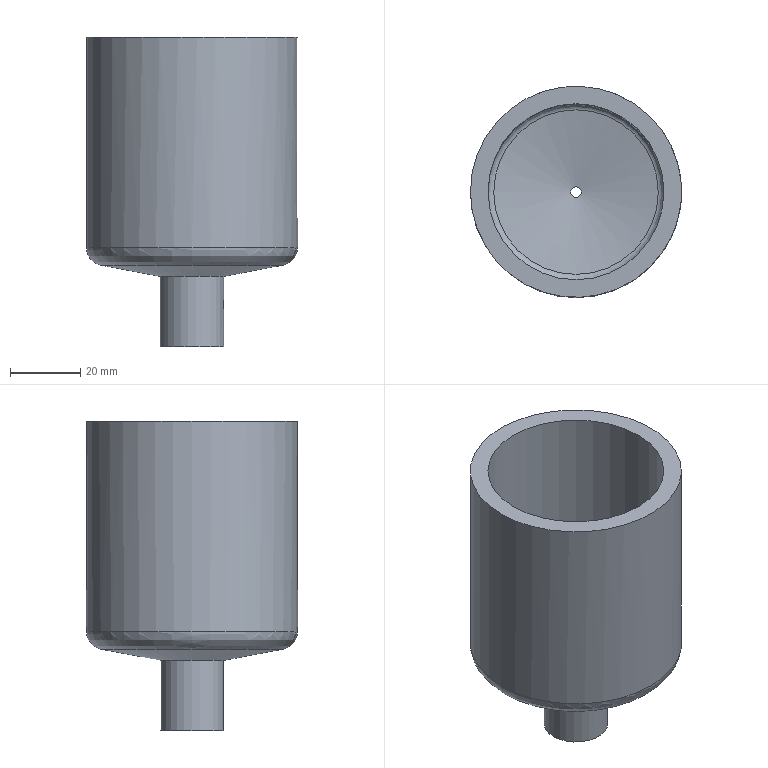Part | NX | features CYLINDER 3, BLEND 2, DATUM_CSYS 2, HOLE PACKAGE 2, SIMPLE HOLE 2, SYMBOLIC_THREAD 2, SKETCH 1, SWP104 1 | 1 solid | 18 faces | box 60 x 60 x 88 mm | volume 68833 mm3 | cylinder 8 | cone 4 | plane 4 | torus 2 | commonest cylinder face diameters 3 x2 8.5 x1 8.7 x1 12 x1 18 x1 50 x1
STEP:
#1=CARTESIAN_POINT('',(30.,0.,28.138));
#2=VERTEX_POINT('',#1);
#3=CARTESIAN_POINT('',(0.,0.,28.138));
#4=DIRECTION('',(0.,0.,1.));
#5=DIRECTION('',(1.,0.,0.));
#6=AXIS2_PLACEMENT_3D('',#3,#4,#5);
#7=CIRCLE('',#6,30.);
#8=EDGE_CURVE('',#2,#2,#7,.T.);
#9=ORIENTED_EDGE('',*,*,#8,.T.);
#10=EDGE_LOOP('',(#9));
#11=FACE_BOUND('',#10,.T.);
#12=CARTESIAN_POINT('',(-30.,0.,88.));
#13=VERTEX_POINT('',#12);
#14=CARTESIAN_POINT('',(0.,0.,88.));
#15=DIRECTION('',(0.,0.,-1.));
#16=DIRECTION('',(-1.,0.,0.));
#17=AXIS2_PLACEMENT_3D('',#14,#15,#16);
#18=CIRCLE('',#17,30.);
#19=EDGE_CURVE('',#13,#13,#18,.T.);
#20=ORIENTED_EDGE('',*,*,#19,.T.);
#21=EDGE_LOOP('',(#20));
#22=FACE_BOUND('',#21,.T.);
#23=CARTESIAN_POINT('',(0.,0.,0.));
#24=DIRECTION('',(0.,0.,-1.));
#25=DIRECTION('',(-1.,0.,0.));
#26=AXIS2_PLACEMENT_3D('',#23,#24,#25);
#27=CYLINDRICAL_SURFACE('',#26,30.);
#28=ADVANCED_FACE('',(#11,#22),#27,.T.);
#29=CARTESIAN_POINT('',(-25.936,0.,23.226));
#30=VERTEX_POINT('',#29);
#31=CARTESIAN_POINT('',(0.,0.,23.226));
#32=DIRECTION('',(0.,0.,-1.));
#33=DIRECTION('',(-1.,0.,0.));
#34=AXIS2_PLACEMENT_3D('',#31,#32,#33);
#35=CIRCLE('',#34,25.936);
#36=EDGE_CURVE('',#30,#30,#35,.T.);
#37=ORIENTED_EDGE('',*,*,#36,.T.);
#38=EDGE_LOOP('',(#37));
#39=FACE_BOUND('',#38,.T.);
#40=CARTESIAN_POINT('',(-9.,0.,20.));
#41=VERTEX_POINT('',#40);
#42=CARTESIAN_POINT('',(0.,0.,20.));
#43=DIRECTION('',(0.,0.,-1.));
#44=DIRECTION('',(-1.,0.,0.));
#45=AXIS2_PLACEMENT_3D('',#42,#43,#44);
#46=CIRCLE('',#45,9.);
#47=EDGE_CURVE('',#41,#41,#46,.T.);
#48=ORIENTED_EDGE('',*,*,#47,.F.);
#49=EDGE_LOOP('',(#48));
#50=FACE_BOUND('',#49,.T.);
#51=CARTESIAN_POINT('',(0.,0.,24.));
#52=DIRECTION('',(0.,0.,1.));
#53=DIRECTION('',(1.,0.,0.));
#54=AXIS2_PLACEMENT_3D('',#51,#52,#53);
#55=CONICAL_SURFACE('',#54,30.,1.383);
#56=ADVANCED_FACE('',(#39,#50),#55,.T.);
#57=CARTESIAN_POINT('',(9.,0.,10.5));
#58=VERTEX_POINT('',#57);
#59=CARTESIAN_POINT('',(8.937,1.177,10.826));
#60=CARTESIAN_POINT('',(9.031,-0.0002785,10.337));
#61=CARTESIAN_POINT('',(8.937,-1.176,10.825));
#62=CARTESIAN_POINT('',(8.842,-1.662,11.999));
#63=CARTESIAN_POINT('',(8.937,-1.176,13.175));
#64=CARTESIAN_POINT('',(9.031,-0.00044,13.662));
#65=CARTESIAN_POINT('',(8.938,1.174,13.177));
#66=CARTESIAN_POINT('',(8.842,1.662,12.001));
#67=CARTESIAN_POINT('',(8.937,1.177,10.826));
#68=CARTESIAN_POINT('',(9.031,-0.0002785,10.337));
#69=CARTESIAN_POINT('',(8.937,-1.176,10.825));
#70=B_SPLINE_CURVE_WITH_KNOTS('',3,(#59,#60,#61,#62,#63,#64,#65,#66,#67,#68,#69),.UNSPECIFIED.,.T.,.F.,(1,1,1,1,1,1,1,1,1,1,1,1,1,1,1),(-0.003523,-0.002349,-0.001174,0.,0.001174,0.002349,0.003523,0.004697,0.005872,0.007046,0.00822,0.009395,0.01057,0.01174,0.01292),.UNSPECIFIED.);
#71=EDGE_CURVE('',#58,#58,#70,.T.);
#72=ORIENTED_EDGE('',*,*,#71,.T.);
#73=EDGE_LOOP('',(#72));
#74=FACE_BOUND('',#73,.T.);
#75=CARTESIAN_POINT('',(-9.,0.,0.));
#76=VERTEX_POINT('',#75);
#77=CARTESIAN_POINT('',(0.,0.,0.));
#78=DIRECTION('',(0.,0.,-1.));
#79=DIRECTION('',(-1.,0.,0.));
#80=AXIS2_PLACEMENT_3D('',#77,#78,#79);
#81=CIRCLE('',#80,9.);
#82=EDGE_CURVE('',#76,#76,#81,.T.);
#83=ORIENTED_EDGE('',*,*,#82,.F.);
#84=EDGE_LOOP('',(#83));
#85=FACE_BOUND('',#84,.T.);
#86=ORIENTED_EDGE('',*,*,#47,.T.);
#87=EDGE_LOOP('',(#86));
#88=FACE_BOUND('',#87,.T.);
#89=CARTESIAN_POINT('',(0.,0.,0.));
#90=DIRECTION('',(0.,0.,-1.));
#91=DIRECTION('',(-1.,0.,0.));
#92=AXIS2_PLACEMENT_3D('',#89,#90,#91);
#93=CYLINDRICAL_SURFACE('',#92,9.);
#94=ADVANCED_FACE('',(#74,#85,#88),#93,.T.);
#95=CARTESIAN_POINT('',(5.,0.,0.));
#96=VERTEX_POINT('',#95);
#97=CARTESIAN_POINT('',(0.,0.,0.));
#98=DIRECTION('',(0.,0.,1.));
#99=DIRECTION('',(1.,0.,0.));
#100=AXIS2_PLACEMENT_3D('',#97,#98,#99);
#101=CIRCLE('',#100,5.);
#102=EDGE_CURVE('',#96,#96,#101,.T.);
#103=ORIENTED_EDGE('',*,*,#102,.T.);
#104=EDGE_LOOP('',(#103));
#105=FACE_BOUND('',#104,.T.);
#106=ORIENTED_EDGE('',*,*,#82,.T.);
#107=EDGE_LOOP('',(#106));
#108=FACE_BOUND('',#107,.T.);
#109=CARTESIAN_POINT('',(0.,9.,0.));
#110=DIRECTION('',(0.,0.,1.));
#111=DIRECTION('',(1.,0.,0.));
#112=AXIS2_PLACEMENT_3D('',#109,#110,#111);
#113=PLANE('',#112);
#114=ADVANCED_FACE('',(#105,#108),#113,.F.);
#115=CARTESIAN_POINT('',(23.374,0.,27.828));
#116=VERTEX_POINT('',#115);
#117=CARTESIAN_POINT('',(0.,0.,27.828));
#118=DIRECTION('',(0.,0.,1.));
#119=DIRECTION('',(1.,0.,0.));
#120=AXIS2_PLACEMENT_3D('',#117,#118,#119);
#121=CIRCLE('',#120,23.374);
#122=EDGE_CURVE('',#116,#116,#121,.T.);
#123=ORIENTED_EDGE('',*,*,#122,.T.);
#124=EDGE_LOOP('',(#123));
#125=FACE_BOUND('',#124,.T.);
#126=CARTESIAN_POINT('',(1.5,0.,23.661));
#127=VERTEX_POINT('',#126);
#128=CARTESIAN_POINT('',(0.,0.,23.661));
#129=DIRECTION('',(0.,0.,1.));
#130=DIRECTION('',(1.,0.,0.));
#131=AXIS2_PLACEMENT_3D('',#128,#129,#130);
#132=CIRCLE('',#131,1.5);
#133=EDGE_CURVE('',#127,#127,#132,.F.);
#134=ORIENTED_EDGE('',*,*,#133,.T.);
#135=EDGE_LOOP('',(#134));
#136=FACE_BOUND('',#135,.T.);
#137=CARTESIAN_POINT('',(0.,0.,23.376));
#138=DIRECTION('',(0.,0.,1.));
#139=DIRECTION('',(1.,0.,0.));
#140=AXIS2_PLACEMENT_3D('',#137,#138,#139);
#141=CONICAL_SURFACE('',#140,0.,1.383);
#142=ADVANCED_FACE('',(#125,#136),#141,.F.);
#143=CARTESIAN_POINT('',(-25.,0.,29.793));
#144=VERTEX_POINT('',#143);
#145=CARTESIAN_POINT('',(0.,0.,29.793));
#146=DIRECTION('',(0.,0.,-1.));
#147=DIRECTION('',(-1.,0.,0.));
#148=AXIS2_PLACEMENT_3D('',#145,#146,#147);
#149=CIRCLE('',#148,25.);
#150=EDGE_CURVE('',#144,#144,#149,.T.);
#151=ORIENTED_EDGE('',*,*,#150,.T.);
#152=EDGE_LOOP('',(#151));
#153=FACE_BOUND('',#152,.T.);
#154=CARTESIAN_POINT('',(-25.,0.,88.));
#155=VERTEX_POINT('',#154);
#156=CARTESIAN_POINT('',(0.,0.,88.));
#157=DIRECTION('',(0.,0.,-1.));
#158=DIRECTION('',(-1.,0.,0.));
#159=AXIS2_PLACEMENT_3D('',#156,#157,#158);
#160=CIRCLE('',#159,25.);
#161=EDGE_CURVE('',#155,#155,#160,.T.);
#162=ORIENTED_EDGE('',*,*,#161,.F.);
#163=EDGE_LOOP('',(#162));
#164=FACE_BOUND('',#163,.T.);
#165=CARTESIAN_POINT('',(0.,0.,0.));
#166=DIRECTION('',(0.,0.,-1.));
#167=DIRECTION('',(-1.,0.,0.));
#168=AXIS2_PLACEMENT_3D('',#165,#166,#167);
#169=CYLINDRICAL_SURFACE('',#168,25.);
#170=ADVANCED_FACE('',(#153,#164),#169,.F.);
#171=ORIENTED_EDGE('',*,*,#19,.F.);
#172=EDGE_LOOP('',(#171));
#173=FACE_BOUND('',#172,.T.);
#174=ORIENTED_EDGE('',*,*,#161,.T.);
#175=EDGE_LOOP('',(#174));
#176=FACE_BOUND('',#175,.T.);
#177=CARTESIAN_POINT('',(0.,25.,88.));
#178=DIRECTION('',(0.,0.,-1.));
#179=DIRECTION('',(-1.,0.,0.));
#180=AXIS2_PLACEMENT_3D('',#177,#178,#179);
#181=PLANE('',#180);
#182=ADVANCED_FACE('',(#173,#176),#181,.F.);
#183=CARTESIAN_POINT('',(4.25,0.,0.75));
#184=VERTEX_POINT('',#183);
#185=CARTESIAN_POINT('',(0.,0.,0.75));
#186=DIRECTION('',(0.,0.,1.));
#187=DIRECTION('',(1.,0.,0.));
#188=AXIS2_PLACEMENT_3D('',#185,#186,#187);
#189=CIRCLE('',#188,4.25);
#190=EDGE_CURVE('',#184,#184,#189,.F.);
#191=ORIENTED_EDGE('',*,*,#190,.T.);
#192=EDGE_LOOP('',(#191));
#193=FACE_BOUND('',#192,.T.);
#194=CARTESIAN_POINT('',(-4.25,0.,10.));
#195=VERTEX_POINT('',#194);
#196=CARTESIAN_POINT('',(0.,0.,10.));
#197=DIRECTION('',(0.,0.,-1.));
#198=DIRECTION('',(-1.,0.,0.));
#199=AXIS2_PLACEMENT_3D('',#196,#197,#198);
#200=CIRCLE('',#199,4.25);
#201=EDGE_CURVE('',#195,#195,#200,.F.);
#202=ORIENTED_EDGE('',*,*,#201,.T.);
#203=EDGE_LOOP('',(#202));
#204=FACE_BOUND('',#203,.T.);
#205=CARTESIAN_POINT('',(0.,0.,0.));
#206=DIRECTION('',(0.,0.,1.));
#207=DIRECTION('',(1.,0.,0.));
#208=AXIS2_PLACEMENT_3D('',#205,#206,#207);
#209=CYLINDRICAL_SURFACE('',#208,4.25);
#210=ADVANCED_FACE('',(#193,#204),#209,.F.);
#211=ORIENTED_EDGE('',*,*,#190,.F.);
#212=EDGE_LOOP('',(#211));
#213=FACE_BOUND('',#212,.T.);
#214=ORIENTED_EDGE('',*,*,#102,.F.);
#215=EDGE_LOOP('',(#214));
#216=FACE_BOUND('',#215,.T.);
#217=CARTESIAN_POINT('',(0.,0.,0.));
#218=DIRECTION('',(0.,0.,-1.));
#219=DIRECTION('',(-1.,0.,0.));
#220=AXIS2_PLACEMENT_3D('',#217,#218,#219);
#221=CONICAL_SURFACE('',#220,5.,0.7854);
#222=ADVANCED_FACE('',(#213,#216),#221,.F.);
#223=CARTESIAN_POINT('',(6.,0.,10.));
#224=VERTEX_POINT('',#223);
#225=CARTESIAN_POINT('',(0.,0.,10.));
#226=DIRECTION('',(0.,0.,1.));
#227=DIRECTION('',(1.,0.,0.));
#228=AXIS2_PLACEMENT_3D('',#225,#226,#227);
#229=CIRCLE('',#228,6.);
#230=EDGE_CURVE('',#224,#224,#229,.T.);
#231=ORIENTED_EDGE('',*,*,#230,.T.);
#232=EDGE_LOOP('',(#231));
#233=FACE_BOUND('',#232,.T.);
#234=ORIENTED_EDGE('',*,*,#201,.F.);
#235=EDGE_LOOP('',(#234));
#236=FACE_BOUND('',#235,.T.);
#237=CARTESIAN_POINT('',(0.,0.,10.));
#238=DIRECTION('',(0.,0.,-1.));
#239=DIRECTION('',(-1.,0.,0.));
#240=AXIS2_PLACEMENT_3D('',#237,#238,#239);
#241=PLANE('',#240);
#242=ADVANCED_FACE('',(#233,#236),#241,.F.);
#243=CARTESIAN_POINT('',(4.35,0.,14.));
#244=VERTEX_POINT('',#243);
#245=CARTESIAN_POINT('',(0.,0.,14.));
#246=DIRECTION('',(0.,0.,1.));
#247=DIRECTION('',(1.,0.,0.));
#248=AXIS2_PLACEMENT_3D('',#245,#246,#247);
#249=CIRCLE('',#248,4.35);
#250=EDGE_CURVE('',#244,#244,#249,.T.);
#251=ORIENTED_EDGE('',*,*,#250,.T.);
#252=EDGE_LOOP('',(#251));
#253=FACE_BOUND('',#252,.T.);
#254=CARTESIAN_POINT('',(-6.,0.,14.));
#255=VERTEX_POINT('',#254);
#256=CARTESIAN_POINT('',(0.,0.,14.));
#257=DIRECTION('',(0.,0.,-1.));
#258=DIRECTION('',(-1.,0.,0.));
#259=AXIS2_PLACEMENT_3D('',#256,#257,#258);
#260=CIRCLE('',#259,6.);
#261=EDGE_CURVE('',#255,#255,#260,.T.);
#262=ORIENTED_EDGE('',*,*,#261,.T.);
#263=EDGE_LOOP('',(#262));
#264=FACE_BOUND('',#263,.T.);
#265=CARTESIAN_POINT('',(0.,0.,14.));
#266=DIRECTION('',(0.,0.,1.));
#267=DIRECTION('',(1.,0.,0.));
#268=AXIS2_PLACEMENT_3D('',#265,#266,#267);
#269=PLANE('',#268);
#270=ADVANCED_FACE('',(#253,#264),#269,.F.);
#271=CARTESIAN_POINT('',(6.,0.,10.5));
#272=VERTEX_POINT('',#271);
#273=CARTESIAN_POINT('',(5.906,-1.177,10.826));
#274=CARTESIAN_POINT('',(6.047,0.0002147,10.337));
#275=CARTESIAN_POINT('',(5.906,1.176,10.825));
#276=CARTESIAN_POINT('',(5.761,1.662,11.998));
#277=CARTESIAN_POINT('',(5.906,1.175,13.176));
#278=CARTESIAN_POINT('',(6.047,0.0007133,13.662));
#279=CARTESIAN_POINT('',(5.906,-1.174,13.176));
#280=CARTESIAN_POINT('',(5.761,-1.662,12.001));
#281=CARTESIAN_POINT('',(5.906,-1.177,10.826));
#282=CARTESIAN_POINT('',(6.047,0.0002147,10.337));
#283=CARTESIAN_POINT('',(5.906,1.176,10.825));
#284=B_SPLINE_CURVE_WITH_KNOTS('',3,(#273,#274,#275,#276,#277,#278,#279,#280,#281,#282,#283),.UNSPECIFIED.,.T.,.F.,(1,1,1,1,1,1,1,1,1,1,1,1,1,1,1),(-0.003531,-0.002354,-0.001177,0.,0.001177,0.002354,0.003531,0.004708,0.005885,0.007062,0.008239,0.009416,0.01059,0.01177,0.01295),.UNSPECIFIED.);
#285=EDGE_CURVE('',#272,#272,#284,.T.);
#286=ORIENTED_EDGE('',*,*,#285,.T.);
#287=EDGE_LOOP('',(#286));
#288=FACE_BOUND('',#287,.T.);
#289=ORIENTED_EDGE('',*,*,#261,.F.);
#290=EDGE_LOOP('',(#289));
#291=FACE_BOUND('',#290,.T.);
#292=ORIENTED_EDGE('',*,*,#230,.F.);
#293=EDGE_LOOP('',(#292));
#294=FACE_BOUND('',#293,.T.);
#295=CARTESIAN_POINT('',(0.,0.,10.));
#296=DIRECTION('',(0.,0.,1.));
#297=DIRECTION('',(1.,0.,0.));
#298=AXIS2_PLACEMENT_3D('',#295,#296,#297);
#299=CYLINDRICAL_SURFACE('',#298,6.);
#300=ADVANCED_FACE('',(#288,#291,#294),#299,.F.);
#301=CARTESIAN_POINT('',(-1.5,0.,17.645));
#302=VERTEX_POINT('',#301);
#303=CARTESIAN_POINT('',(0.,0.,17.645));
#304=DIRECTION('',(0.,0.,-1.));
#305=DIRECTION('',(-1.,0.,0.));
#306=AXIS2_PLACEMENT_3D('',#303,#304,#305);
#307=CIRCLE('',#306,1.5);
#308=EDGE_CURVE('',#302,#302,#307,.F.);
#309=ORIENTED_EDGE('',*,*,#308,.T.);
#310=EDGE_LOOP('',(#309));
#311=FACE_BOUND('',#310,.T.);
#312=CARTESIAN_POINT('',(4.35,0.,16.));
#313=VERTEX_POINT('',#312);
#314=CARTESIAN_POINT('',(0.,0.,16.));
#315=DIRECTION('',(0.,0.,1.));
#316=DIRECTION('',(1.,0.,0.));
#317=AXIS2_PLACEMENT_3D('',#314,#315,#316);
#318=CIRCLE('',#317,4.35);
#319=EDGE_CURVE('',#313,#313,#318,.T.);
#320=ORIENTED_EDGE('',*,*,#319,.F.);
#321=EDGE_LOOP('',(#320));
#322=FACE_BOUND('',#321,.T.);
#323=CARTESIAN_POINT('',(0.,0.,16.));
#324=DIRECTION('',(0.,0.,-1.));
#325=DIRECTION('',(-1.,0.,0.));
#326=AXIS2_PLACEMENT_3D('',#323,#324,#325);
#327=CONICAL_SURFACE('',#326,4.35,1.047);
#328=ADVANCED_FACE('',(#311,#322),#327,.F.);
#329=ORIENTED_EDGE('',*,*,#319,.T.);
#330=EDGE_LOOP('',(#329));
#331=FACE_BOUND('',#330,.T.);
#332=ORIENTED_EDGE('',*,*,#250,.F.);
#333=EDGE_LOOP('',(#332));
#334=FACE_BOUND('',#333,.T.);
#335=CARTESIAN_POINT('',(0.,0.,14.));
#336=DIRECTION('',(0.,0.,1.));
#337=DIRECTION('',(1.,0.,0.));
#338=AXIS2_PLACEMENT_3D('',#335,#336,#337);
#339=CYLINDRICAL_SURFACE('',#338,4.35);
#340=ADVANCED_FACE('',(#331,#334),#339,.F.);
#341=ORIENTED_EDGE('',*,*,#308,.F.);
#342=EDGE_LOOP('',(#341));
#343=FACE_BOUND('',#342,.T.);
#344=ORIENTED_EDGE('',*,*,#133,.F.);
#345=EDGE_LOOP('',(#344));
#346=FACE_BOUND('',#345,.T.);
#347=CARTESIAN_POINT('',(0.,0.,0.));
#348=DIRECTION('',(0.,0.,1.));
#349=DIRECTION('',(1.,0.,0.));
#350=AXIS2_PLACEMENT_3D('',#347,#348,#349);
#351=CYLINDRICAL_SURFACE('',#350,1.5);
#352=ADVANCED_FACE('',(#343,#346),#351,.F.);
#353=ORIENTED_EDGE('',*,*,#285,.F.);
#354=EDGE_LOOP('',(#353));
#355=FACE_BOUND('',#354,.T.);
#356=ORIENTED_EDGE('',*,*,#71,.F.);
#357=EDGE_LOOP('',(#356));
#358=FACE_BOUND('',#357,.T.);
#359=CARTESIAN_POINT('',(0.,0.,12.));
#360=DIRECTION('',(1.,0.,0.));
#361=DIRECTION('',(0.,0.,-1.));
#362=AXIS2_PLACEMENT_3D('',#359,#360,#361);
#363=CYLINDRICAL_SURFACE('',#362,1.5);
#364=ADVANCED_FACE('',(#355,#358),#363,.F.);
#365=ORIENTED_EDGE('',*,*,#8,.F.);
#366=EDGE_LOOP('',(#365));
#367=FACE_BOUND('',#366,.T.);
#368=ORIENTED_EDGE('',*,*,#36,.F.);
#369=EDGE_LOOP('',(#368));
#370=FACE_BOUND('',#369,.T.);
#371=CARTESIAN_POINT('',(0.,0.,28.138));
#372=DIRECTION('',(0.,0.,1.));
#373=DIRECTION('',(1.,0.,0.));
#374=AXIS2_PLACEMENT_3D('',#371,#372,#373);
#375=TOROIDAL_SURFACE('',#374,25.,5.);
#376=ADVANCED_FACE('',(#367,#370),#375,.T.);
#377=ORIENTED_EDGE('',*,*,#122,.F.);
#378=EDGE_LOOP('',(#377));
#379=FACE_BOUND('',#378,.T.);
#380=ORIENTED_EDGE('',*,*,#150,.F.);
#381=EDGE_LOOP('',(#380));
#382=FACE_BOUND('',#381,.T.);
#383=CARTESIAN_POINT('',(0.,0.,29.793));
#384=DIRECTION('',(0.,0.,-1.));
#385=DIRECTION('',(-1.,0.,0.));
#386=AXIS2_PLACEMENT_3D('',#383,#384,#385);
#387=TOROIDAL_SURFACE('',#386,23.,2.);
#388=ADVANCED_FACE('',(#379,#382),#387,.F.);
#389=CLOSED_SHELL('',(#28,#56,#94,#114,#142,#170,#182,#210,#222,#242,#270,#300,#328,#340,#352,#364,#376,#388));
#390=MANIFOLD_SOLID_BREP('',#389);
#391=(LENGTH_UNIT()NAMED_UNIT(*)SI_UNIT(.MILLI.,.METRE.));
#392=UNCERTAINTY_MEASURE_WITH_UNIT(LENGTH_MEASURE(0.0508),#391,'','');
#393=(NAMED_UNIT(*)PLANE_ANGLE_UNIT()SI_UNIT($,.RADIAN.));
#394=(NAMED_UNIT(*)SI_UNIT($,.STERADIAN.)SOLID_ANGLE_UNIT());
#395=(GEOMETRIC_REPRESENTATION_CONTEXT(3)GLOBAL_UNCERTAINTY_ASSIGNED_CONTEXT((#392))GLOBAL_UNIT_ASSIGNED_CONTEXT((#391,#393,#394))REPRESENTATION_CONTEXT('',''));
#396=ADVANCED_BREP_SHAPE_REPRESENTATION('',(#390),#395);